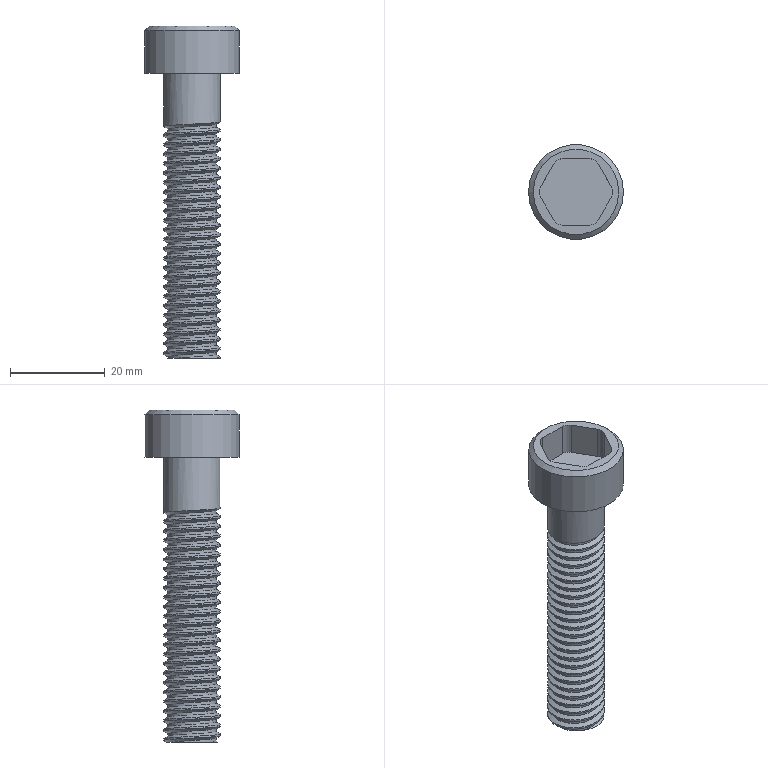Part | NX | features DATUM_CSYS 3, EXTRUDE 2, SKETCH 2, BLEND 1, CHAMFER 1, CYLINDER 1, THREADS 1 | 1 solid | 48 faces | box 20 x 20 x 70 mm | volume 7911 mm3 | cylinder 34 | plane 11 | spline 2 | cone 1 | commonest cylinder face diameters 12 x26 4 x6 10.25 x1 20 x1